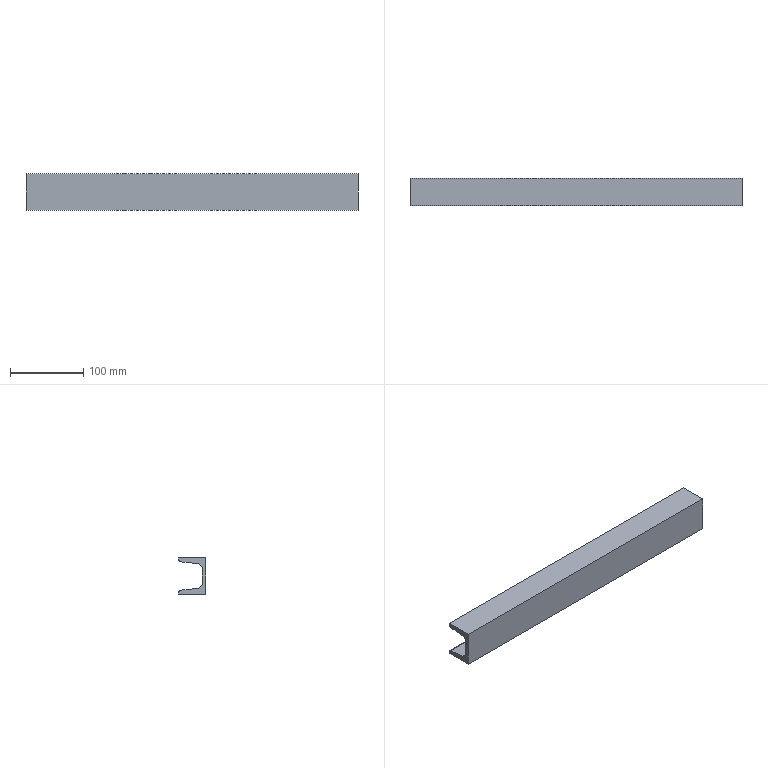Part | SolidWorks | features WeldMemberFeat 1, WeldmentFeature 1 | 1 solid | 14 faces | box 454 x 37 x 50 mm | volume 314305 mm3 | plane 10 | cylinder 4 | commonest cylinder face diameters 7 x2 14 x2
STEP:
#1=CARTESIAN_POINT('',(-227.,33.866,44.379));
#2=VERTEX_POINT('',#1);
#3=CARTESIAN_POINT('',(-227.,37.,47.859));
#4=VERTEX_POINT('',#3);
#5=CARTESIAN_POINT('',(-227.,33.5,47.859));
#6=DIRECTION('',(1.,0.,0.));
#7=DIRECTION('',(0.,1.,0.));
#8=AXIS2_PLACEMENT_3D('',#5,#6,#7);
#9=CIRCLE('',#8,3.5);
#10=EDGE_CURVE('',#2,#4,#9,.T.);
#11=ORIENTED_EDGE('',*,*,#10,.T.);
#12=CARTESIAN_POINT('',(227.,37.,47.859));
#13=VERTEX_POINT('',#12);
#14=CARTESIAN_POINT('',(227.,37.,47.859));
#15=DIRECTION('',(-1.,0.,0.));
#16=VECTOR('',#15,1000.);
#17=LINE('',#14,#16);
#18=EDGE_CURVE('',#13,#4,#17,.T.);
#19=ORIENTED_EDGE('',*,*,#18,.F.);
#20=CARTESIAN_POINT('',(227.,33.866,44.379));
#21=VERTEX_POINT('',#20);
#22=CARTESIAN_POINT('',(227.,33.5,47.859));
#23=DIRECTION('',(1.,0.,0.));
#24=DIRECTION('',(0.,1.,0.));
#25=AXIS2_PLACEMENT_3D('',#22,#23,#24);
#26=CIRCLE('',#25,3.5);
#27=EDGE_CURVE('',#21,#13,#26,.T.);
#28=ORIENTED_EDGE('',*,*,#27,.F.);
#29=CARTESIAN_POINT('',(227.,33.866,44.379));
#30=DIRECTION('',(-1.,0.,0.));
#31=VECTOR('',#30,1000.);
#32=LINE('',#29,#31);
#33=EDGE_CURVE('',#21,#2,#32,.T.);
#34=ORIENTED_EDGE('',*,*,#33,.T.);
#35=EDGE_LOOP('',(#11,#19,#28,#34));
#36=FACE_OUTER_BOUND('',#35,.T.);
#37=CARTESIAN_POINT('',(227.,33.5,47.859));
#38=DIRECTION('',(-1.,0.,0.));
#39=DIRECTION('',(0.,-1.,0.));
#40=AXIS2_PLACEMENT_3D('',#37,#38,#39);
#41=CYLINDRICAL_SURFACE('',#40,3.5);
#42=ADVANCED_FACE('',(#36),#41,.T.);
#43=CARTESIAN_POINT('',(-227.,37.,50.));
#44=VERTEX_POINT('',#43);
#45=CARTESIAN_POINT('',(-227.,37.,50.));
#46=DIRECTION('',(0.,0.,1.));
#47=VECTOR('',#46,1000.);
#48=LINE('',#45,#47);
#49=EDGE_CURVE('',#4,#44,#48,.T.);
#50=ORIENTED_EDGE('',*,*,#49,.T.);
#51=CARTESIAN_POINT('',(227.,37.,50.));
#52=VERTEX_POINT('',#51);
#53=CARTESIAN_POINT('',(227.,37.,50.));
#54=DIRECTION('',(-1.,0.,0.));
#55=VECTOR('',#54,1000.);
#56=LINE('',#53,#55);
#57=EDGE_CURVE('',#52,#44,#56,.T.);
#58=ORIENTED_EDGE('',*,*,#57,.F.);
#59=CARTESIAN_POINT('',(227.,37.,50.));
#60=DIRECTION('',(0.,0.,1.));
#61=VECTOR('',#60,1000.);
#62=LINE('',#59,#61);
#63=EDGE_CURVE('',#13,#52,#62,.T.);
#64=ORIENTED_EDGE('',*,*,#63,.F.);
#65=ORIENTED_EDGE('',*,*,#18,.T.);
#66=EDGE_LOOP('',(#50,#58,#64,#65));
#67=FACE_OUTER_BOUND('',#66,.T.);
#68=CARTESIAN_POINT('',(227.,37.,50.));
#69=DIRECTION('',(0.,-1.,0.));
#70=DIRECTION('',(1.,0.,0.));
#71=AXIS2_PLACEMENT_3D('',#68,#69,#70);
#72=PLANE('',#71);
#73=ADVANCED_FACE('',(#67),#72,.F.);
#74=CARTESIAN_POINT('',(-227.,0.,50.));
#75=VERTEX_POINT('',#74);
#76=CARTESIAN_POINT('',(-227.,37.,50.));
#77=DIRECTION('',(0.,-1.,0.));
#78=VECTOR('',#77,1000.);
#79=LINE('',#76,#78);
#80=EDGE_CURVE('',#44,#75,#79,.T.);
#81=ORIENTED_EDGE('',*,*,#80,.T.);
#82=CARTESIAN_POINT('',(227.,0.,50.));
#83=VERTEX_POINT('',#82);
#84=CARTESIAN_POINT('',(227.,0.,50.));
#85=DIRECTION('',(-1.,0.,0.));
#86=VECTOR('',#85,1000.);
#87=LINE('',#84,#86);
#88=EDGE_CURVE('',#83,#75,#87,.T.);
#89=ORIENTED_EDGE('',*,*,#88,.F.);
#90=CARTESIAN_POINT('',(227.,37.,50.));
#91=DIRECTION('',(0.,-1.,0.));
#92=VECTOR('',#91,1000.);
#93=LINE('',#90,#92);
#94=EDGE_CURVE('',#52,#83,#93,.T.);
#95=ORIENTED_EDGE('',*,*,#94,.F.);
#96=ORIENTED_EDGE('',*,*,#57,.T.);
#97=EDGE_LOOP('',(#81,#89,#95,#96));
#98=FACE_OUTER_BOUND('',#97,.T.);
#99=CARTESIAN_POINT('',(227.,37.,50.));
#100=DIRECTION('',(0.,0.,-1.));
#101=DIRECTION('',(0.,1.,0.));
#102=AXIS2_PLACEMENT_3D('',#99,#100,#101);
#103=PLANE('',#102);
#104=ADVANCED_FACE('',(#98),#103,.F.);
#105=CARTESIAN_POINT('',(-227.,0.,0.));
#106=VERTEX_POINT('',#105);
#107=CARTESIAN_POINT('',(-227.,0.,50.));
#108=DIRECTION('',(0.,0.,-1.));
#109=VECTOR('',#108,1000.);
#110=LINE('',#107,#109);
#111=EDGE_CURVE('',#75,#106,#110,.T.);
#112=ORIENTED_EDGE('',*,*,#111,.T.);
#113=CARTESIAN_POINT('',(227.,0.,0.));
#114=VERTEX_POINT('',#113);
#115=CARTESIAN_POINT('',(227.,0.,0.));
#116=DIRECTION('',(-1.,0.,0.));
#117=VECTOR('',#116,1000.);
#118=LINE('',#115,#117);
#119=EDGE_CURVE('',#114,#106,#118,.T.);
#120=ORIENTED_EDGE('',*,*,#119,.F.);
#121=CARTESIAN_POINT('',(227.,0.,50.));
#122=DIRECTION('',(0.,0.,-1.));
#123=VECTOR('',#122,1000.);
#124=LINE('',#121,#123);
#125=EDGE_CURVE('',#83,#114,#124,.T.);
#126=ORIENTED_EDGE('',*,*,#125,.F.);
#127=ORIENTED_EDGE('',*,*,#88,.T.);
#128=EDGE_LOOP('',(#112,#120,#126,#127));
#129=FACE_OUTER_BOUND('',#128,.T.);
#130=CARTESIAN_POINT('',(227.,0.,50.));
#131=DIRECTION('',(0.,1.,0.));
#132=DIRECTION('',(-1.,0.,0.));
#133=AXIS2_PLACEMENT_3D('',#130,#131,#132);
#134=PLANE('',#133);
#135=ADVANCED_FACE('',(#129),#134,.F.);
#136=CARTESIAN_POINT('',(-227.,37.,0.));
#137=VERTEX_POINT('',#136);
#138=CARTESIAN_POINT('',(-227.,37.,0.));
#139=DIRECTION('',(0.,1.,0.));
#140=VECTOR('',#139,1000.);
#141=LINE('',#138,#140);
#142=EDGE_CURVE('',#106,#137,#141,.T.);
#143=ORIENTED_EDGE('',*,*,#142,.T.);
#144=CARTESIAN_POINT('',(227.,37.,0.));
#145=VERTEX_POINT('',#144);
#146=CARTESIAN_POINT('',(227.,37.,0.));
#147=DIRECTION('',(-1.,0.,0.));
#148=VECTOR('',#147,1000.);
#149=LINE('',#146,#148);
#150=EDGE_CURVE('',#145,#137,#149,.T.);
#151=ORIENTED_EDGE('',*,*,#150,.F.);
#152=CARTESIAN_POINT('',(227.,37.,0.));
#153=DIRECTION('',(0.,1.,0.));
#154=VECTOR('',#153,1000.);
#155=LINE('',#152,#154);
#156=EDGE_CURVE('',#114,#145,#155,.T.);
#157=ORIENTED_EDGE('',*,*,#156,.F.);
#158=ORIENTED_EDGE('',*,*,#119,.T.);
#159=EDGE_LOOP('',(#143,#151,#157,#158));
#160=FACE_OUTER_BOUND('',#159,.T.);
#161=CARTESIAN_POINT('',(227.,37.,0.));
#162=DIRECTION('',(0.,0.,1.));
#163=DIRECTION('',(0.,-1.,0.));
#164=AXIS2_PLACEMENT_3D('',#161,#162,#163);
#165=PLANE('',#164);
#166=ADVANCED_FACE('',(#160),#165,.F.);
#167=CARTESIAN_POINT('',(-227.,37.,2.141));
#168=VERTEX_POINT('',#167);
#169=CARTESIAN_POINT('',(-227.,37.,0.));
#170=DIRECTION('',(0.,0.,1.));
#171=VECTOR('',#170,1000.);
#172=LINE('',#169,#171);
#173=EDGE_CURVE('',#137,#168,#172,.T.);
#174=ORIENTED_EDGE('',*,*,#173,.T.);
#175=CARTESIAN_POINT('',(227.,37.,2.141));
#176=VERTEX_POINT('',#175);
#177=CARTESIAN_POINT('',(227.,37.,2.141));
#178=DIRECTION('',(-1.,0.,0.));
#179=VECTOR('',#178,1000.);
#180=LINE('',#177,#179);
#181=EDGE_CURVE('',#176,#168,#180,.T.);
#182=ORIENTED_EDGE('',*,*,#181,.F.);
#183=CARTESIAN_POINT('',(227.,37.,0.));
#184=DIRECTION('',(0.,0.,1.));
#185=VECTOR('',#184,1000.);
#186=LINE('',#183,#185);
#187=EDGE_CURVE('',#145,#176,#186,.T.);
#188=ORIENTED_EDGE('',*,*,#187,.F.);
#189=ORIENTED_EDGE('',*,*,#150,.T.);
#190=EDGE_LOOP('',(#174,#182,#188,#189));
#191=FACE_OUTER_BOUND('',#190,.T.);
#192=CARTESIAN_POINT('',(227.,37.,0.));
#193=DIRECTION('',(0.,-1.,0.));
#194=DIRECTION('',(1.,0.,0.));
#195=AXIS2_PLACEMENT_3D('',#192,#193,#194);
#196=PLANE('',#195);
#197=ADVANCED_FACE('',(#191),#196,.F.);
#198=CARTESIAN_POINT('',(-227.,33.866,5.621));
#199=VERTEX_POINT('',#198);
#200=CARTESIAN_POINT('',(-227.,33.5,2.141));
#201=DIRECTION('',(1.,0.,0.));
#202=DIRECTION('',(0.,-1.,0.));
#203=AXIS2_PLACEMENT_3D('',#200,#201,#202);
#204=CIRCLE('',#203,3.5);
#205=EDGE_CURVE('',#168,#199,#204,.T.);
#206=ORIENTED_EDGE('',*,*,#205,.T.);
#207=CARTESIAN_POINT('',(227.,33.866,5.621));
#208=VERTEX_POINT('',#207);
#209=CARTESIAN_POINT('',(227.,33.866,5.621));
#210=DIRECTION('',(-1.,0.,0.));
#211=VECTOR('',#210,1000.);
#212=LINE('',#209,#211);
#213=EDGE_CURVE('',#208,#199,#212,.T.);
#214=ORIENTED_EDGE('',*,*,#213,.F.);
#215=CARTESIAN_POINT('',(227.,33.5,2.141));
#216=DIRECTION('',(1.,0.,0.));
#217=DIRECTION('',(0.,-1.,0.));
#218=AXIS2_PLACEMENT_3D('',#215,#216,#217);
#219=CIRCLE('',#218,3.5);
#220=EDGE_CURVE('',#176,#208,#219,.T.);
#221=ORIENTED_EDGE('',*,*,#220,.F.);
#222=ORIENTED_EDGE('',*,*,#181,.T.);
#223=EDGE_LOOP('',(#206,#214,#221,#222));
#224=FACE_OUTER_BOUND('',#223,.T.);
#225=CARTESIAN_POINT('',(227.,33.5,2.141));
#226=DIRECTION('',(-1.,0.,0.));
#227=DIRECTION('',(0.,-1.,0.));
#228=AXIS2_PLACEMENT_3D('',#225,#226,#227);
#229=CYLINDRICAL_SURFACE('',#228,3.5);
#230=ADVANCED_FACE('',(#224),#229,.T.);
#231=CARTESIAN_POINT('',(-227.,10.768,8.049));
#232=VERTEX_POINT('',#231);
#233=CARTESIAN_POINT('',(-227.,10.768,8.049));
#234=DIRECTION('',(0.,-0.9945,0.1045));
#235=VECTOR('',#234,1000.);
#236=LINE('',#233,#235);
#237=EDGE_CURVE('',#199,#232,#236,.T.);
#238=ORIENTED_EDGE('',*,*,#237,.T.);
#239=CARTESIAN_POINT('',(227.,10.768,8.049));
#240=VERTEX_POINT('',#239);
#241=CARTESIAN_POINT('',(227.,10.768,8.049));
#242=DIRECTION('',(-1.,0.,0.));
#243=VECTOR('',#242,1000.);
#244=LINE('',#241,#243);
#245=EDGE_CURVE('',#240,#232,#244,.T.);
#246=ORIENTED_EDGE('',*,*,#245,.F.);
#247=CARTESIAN_POINT('',(227.,10.768,8.049));
#248=DIRECTION('',(0.,-0.9945,0.1045));
#249=VECTOR('',#248,1000.);
#250=LINE('',#247,#249);
#251=EDGE_CURVE('',#208,#240,#250,.T.);
#252=ORIENTED_EDGE('',*,*,#251,.F.);
#253=ORIENTED_EDGE('',*,*,#213,.T.);
#254=EDGE_LOOP('',(#238,#246,#252,#253));
#255=FACE_OUTER_BOUND('',#254,.T.);
#256=CARTESIAN_POINT('',(227.,10.768,8.049));
#257=DIRECTION('',(0.,-0.1045,-0.9945));
#258=DIRECTION('',(0.,0.9945,-0.1045));
#259=AXIS2_PLACEMENT_3D('',#256,#257,#258);
#260=PLANE('',#259);
#261=ADVANCED_FACE('',(#255),#260,.F.);
#262=CARTESIAN_POINT('',(-227.,4.5,15.011));
#263=VERTEX_POINT('',#262);
#264=CARTESIAN_POINT('',(-227.,11.5,15.011));
#265=DIRECTION('',(-1.,0.,0.));
#266=DIRECTION('',(0.,1.,0.));
#267=AXIS2_PLACEMENT_3D('',#264,#265,#266);
#268=CIRCLE('',#267,7.);
#269=EDGE_CURVE('',#232,#263,#268,.T.);
#270=ORIENTED_EDGE('',*,*,#269,.T.);
#271=CARTESIAN_POINT('',(227.,4.5,15.011));
#272=VERTEX_POINT('',#271);
#273=CARTESIAN_POINT('',(227.,4.5,15.011));
#274=DIRECTION('',(-1.,0.,0.));
#275=VECTOR('',#274,1000.);
#276=LINE('',#273,#275);
#277=EDGE_CURVE('',#272,#263,#276,.T.);
#278=ORIENTED_EDGE('',*,*,#277,.F.);
#279=CARTESIAN_POINT('',(227.,11.5,15.011));
#280=DIRECTION('',(-1.,0.,0.));
#281=DIRECTION('',(0.,1.,0.));
#282=AXIS2_PLACEMENT_3D('',#279,#280,#281);
#283=CIRCLE('',#282,7.);
#284=EDGE_CURVE('',#240,#272,#283,.T.);
#285=ORIENTED_EDGE('',*,*,#284,.F.);
#286=ORIENTED_EDGE('',*,*,#245,.T.);
#287=EDGE_LOOP('',(#270,#278,#285,#286));
#288=FACE_OUTER_BOUND('',#287,.T.);
#289=CARTESIAN_POINT('',(227.,11.5,15.011));
#290=DIRECTION('',(-1.,0.,0.));
#291=DIRECTION('',(0.,-1.,0.));
#292=AXIS2_PLACEMENT_3D('',#289,#290,#291);
#293=CYLINDRICAL_SURFACE('',#292,7.);
#294=ADVANCED_FACE('',(#288),#293,.F.);
#295=CARTESIAN_POINT('',(-227.,4.5,34.989));
#296=VERTEX_POINT('',#295);
#297=CARTESIAN_POINT('',(-227.,4.5,34.989));
#298=DIRECTION('',(0.,0.,1.));
#299=VECTOR('',#298,1000.);
#300=LINE('',#297,#299);
#301=EDGE_CURVE('',#263,#296,#300,.T.);
#302=ORIENTED_EDGE('',*,*,#301,.T.);
#303=CARTESIAN_POINT('',(227.,4.5,34.989));
#304=VERTEX_POINT('',#303);
#305=CARTESIAN_POINT('',(227.,4.5,34.989));
#306=DIRECTION('',(-1.,0.,0.));
#307=VECTOR('',#306,1000.);
#308=LINE('',#305,#307);
#309=EDGE_CURVE('',#304,#296,#308,.T.);
#310=ORIENTED_EDGE('',*,*,#309,.F.);
#311=CARTESIAN_POINT('',(227.,4.5,34.989));
#312=DIRECTION('',(0.,0.,1.));
#313=VECTOR('',#312,1000.);
#314=LINE('',#311,#313);
#315=EDGE_CURVE('',#272,#304,#314,.T.);
#316=ORIENTED_EDGE('',*,*,#315,.F.);
#317=ORIENTED_EDGE('',*,*,#277,.T.);
#318=EDGE_LOOP('',(#302,#310,#316,#317));
#319=FACE_OUTER_BOUND('',#318,.T.);
#320=CARTESIAN_POINT('',(227.,4.5,34.989));
#321=DIRECTION('',(0.,-1.,0.));
#322=DIRECTION('',(1.,0.,0.));
#323=AXIS2_PLACEMENT_3D('',#320,#321,#322);
#324=PLANE('',#323);
#325=ADVANCED_FACE('',(#319),#324,.F.);
#326=CARTESIAN_POINT('',(-227.,10.768,41.951));
#327=VERTEX_POINT('',#326);
#328=CARTESIAN_POINT('',(-227.,11.5,34.989));
#329=DIRECTION('',(-1.,0.,0.));
#330=DIRECTION('',(0.,-1.,0.));
#331=AXIS2_PLACEMENT_3D('',#328,#329,#330);
#332=CIRCLE('',#331,7.);
#333=EDGE_CURVE('',#296,#327,#332,.T.);
#334=ORIENTED_EDGE('',*,*,#333,.T.);
#335=CARTESIAN_POINT('',(227.,10.768,41.951));
#336=VERTEX_POINT('',#335);
#337=CARTESIAN_POINT('',(227.,10.768,41.951));
#338=DIRECTION('',(-1.,0.,0.));
#339=VECTOR('',#338,1000.);
#340=LINE('',#337,#339);
#341=EDGE_CURVE('',#336,#327,#340,.T.);
#342=ORIENTED_EDGE('',*,*,#341,.F.);
#343=CARTESIAN_POINT('',(227.,11.5,34.989));
#344=DIRECTION('',(-1.,0.,0.));
#345=DIRECTION('',(0.,-1.,0.));
#346=AXIS2_PLACEMENT_3D('',#343,#344,#345);
#347=CIRCLE('',#346,7.);
#348=EDGE_CURVE('',#304,#336,#347,.T.);
#349=ORIENTED_EDGE('',*,*,#348,.F.);
#350=ORIENTED_EDGE('',*,*,#309,.T.);
#351=EDGE_LOOP('',(#334,#342,#349,#350));
#352=FACE_OUTER_BOUND('',#351,.T.);
#353=CARTESIAN_POINT('',(227.,11.5,34.989));
#354=DIRECTION('',(-1.,0.,0.));
#355=DIRECTION('',(0.,-1.,0.));
#356=AXIS2_PLACEMENT_3D('',#353,#354,#355);
#357=CYLINDRICAL_SURFACE('',#356,7.);
#358=ADVANCED_FACE('',(#352),#357,.F.);
#359=CARTESIAN_POINT('',(-227.,10.768,41.951));
#360=DIRECTION('',(0.,0.9945,0.1045));
#361=VECTOR('',#360,1000.);
#362=LINE('',#359,#361);
#363=EDGE_CURVE('',#327,#2,#362,.T.);
#364=ORIENTED_EDGE('',*,*,#363,.T.);
#365=ORIENTED_EDGE('',*,*,#33,.F.);
#366=CARTESIAN_POINT('',(227.,10.768,41.951));
#367=DIRECTION('',(0.,0.9945,0.1045));
#368=VECTOR('',#367,1000.);
#369=LINE('',#366,#368);
#370=EDGE_CURVE('',#336,#21,#369,.T.);
#371=ORIENTED_EDGE('',*,*,#370,.F.);
#372=ORIENTED_EDGE('',*,*,#341,.T.);
#373=EDGE_LOOP('',(#364,#365,#371,#372));
#374=FACE_OUTER_BOUND('',#373,.T.);
#375=CARTESIAN_POINT('',(227.,10.768,41.951));
#376=DIRECTION('',(0.,-0.1045,0.9945));
#377=DIRECTION('',(0.,-0.9945,-0.1045));
#378=AXIS2_PLACEMENT_3D('',#375,#376,#377);
#379=PLANE('',#378);
#380=ADVANCED_FACE('',(#374),#379,.F.);
#381=ORIENTED_EDGE('',*,*,#27,.T.);
#382=ORIENTED_EDGE('',*,*,#63,.T.);
#383=ORIENTED_EDGE('',*,*,#94,.T.);
#384=ORIENTED_EDGE('',*,*,#125,.T.);
#385=ORIENTED_EDGE('',*,*,#156,.T.);
#386=ORIENTED_EDGE('',*,*,#187,.T.);
#387=ORIENTED_EDGE('',*,*,#220,.T.);
#388=ORIENTED_EDGE('',*,*,#251,.T.);
#389=ORIENTED_EDGE('',*,*,#284,.T.);
#390=ORIENTED_EDGE('',*,*,#315,.T.);
#391=ORIENTED_EDGE('',*,*,#348,.T.);
#392=ORIENTED_EDGE('',*,*,#370,.T.);
#393=EDGE_LOOP('',(#381,#382,#383,#384,#385,#386,#387,#388,#389,#390,#391,#392));
#394=FACE_OUTER_BOUND('',#393,.T.);
#395=CARTESIAN_POINT('',(227.,33.5,47.859));
#396=DIRECTION('',(1.,0.,0.));
#397=DIRECTION('',(0.,1.,0.));
#398=AXIS2_PLACEMENT_3D('',#395,#396,#397);
#399=PLANE('',#398);
#400=ADVANCED_FACE('',(#394),#399,.T.);
#401=ORIENTED_EDGE('',*,*,#10,.F.);
#402=ORIENTED_EDGE('',*,*,#363,.F.);
#403=ORIENTED_EDGE('',*,*,#333,.F.);
#404=ORIENTED_EDGE('',*,*,#301,.F.);
#405=ORIENTED_EDGE('',*,*,#269,.F.);
#406=ORIENTED_EDGE('',*,*,#237,.F.);
#407=ORIENTED_EDGE('',*,*,#205,.F.);
#408=ORIENTED_EDGE('',*,*,#173,.F.);
#409=ORIENTED_EDGE('',*,*,#142,.F.);
#410=ORIENTED_EDGE('',*,*,#111,.F.);
#411=ORIENTED_EDGE('',*,*,#80,.F.);
#412=ORIENTED_EDGE('',*,*,#49,.F.);
#413=EDGE_LOOP('',(#401,#402,#403,#404,#405,#406,#407,#408,#409,#410,#411,#412));
#414=FACE_OUTER_BOUND('',#413,.T.);
#415=CARTESIAN_POINT('',(-227.,33.5,47.859));
#416=DIRECTION('',(1.,0.,0.));
#417=DIRECTION('',(0.,1.,0.));
#418=AXIS2_PLACEMENT_3D('',#415,#416,#417);
#419=PLANE('',#418);
#420=ADVANCED_FACE('',(#414),#419,.F.);
#421=CLOSED_SHELL('',(#42,#73,#104,#135,#166,#197,#230,#261,#294,#325,#358,#380,#400,#420));
#422=MANIFOLD_SOLID_BREP('',#421);
#423=CARTESIAN_POINT('',(0.,0.,0.));
#424=DIRECTION('',(0.,0.,1.));
#425=DIRECTION('',(1.,0.,0.));
#426=AXIS2_PLACEMENT_3D('',#423,#424,#425);
#427=(LENGTH_UNIT()NAMED_UNIT(*)SI_UNIT(.MILLI.,.METRE.));
#428=UNCERTAINTY_MEASURE_WITH_UNIT(LENGTH_MEASURE(0.00001),#427,'','');
#429=(NAMED_UNIT(*)PLANE_ANGLE_UNIT()SI_UNIT($,.RADIAN.));
#430=(NAMED_UNIT(*)SI_UNIT($,.STERADIAN.)SOLID_ANGLE_UNIT());
#431=(GEOMETRIC_REPRESENTATION_CONTEXT(3)GLOBAL_UNCERTAINTY_ASSIGNED_CONTEXT((#428))GLOBAL_UNIT_ASSIGNED_CONTEXT((#427,#429,#430))REPRESENTATION_CONTEXT('',''));
#432=ADVANCED_BREP_SHAPE_REPRESENTATION('',(#422,#426),#431);